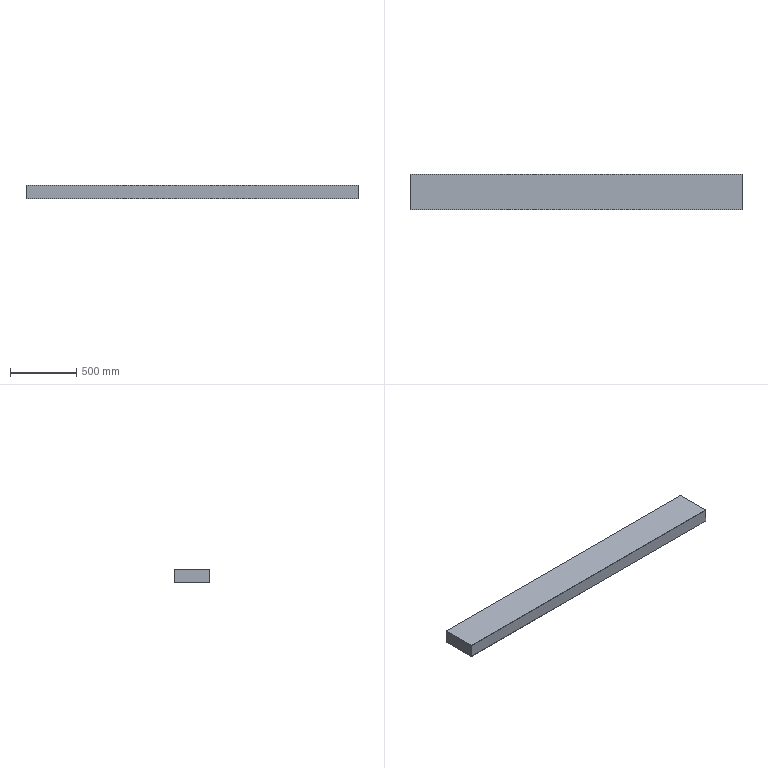Part | STEP file | PN_0037 third-floor site mounting plate 3_Default<As Machined> | 2 solids | 14 faces | box 2515 x 270 x 103 mm | volume 2871750 mm3 | plane 14
STEP:
#1=CARTESIAN_POINT('',(0.,0.,0.));
#2=DIRECTION('',(0.,0.,1.));
#3=DIRECTION('',(1.,0.,0.));
#4=AXIS2_PLACEMENT_3D('',#1,#2,#3);
#5=CARTESIAN_POINT('',(1257.5,-135.,0.));
#6=VERTEX_POINT('',#5);
#7=CARTESIAN_POINT('',(1257.5,135.,0.));
#8=VERTEX_POINT('',#7);
#9=CARTESIAN_POINT('',(1257.5,135.,0.));
#10=DIRECTION('',(0.,1.,0.));
#11=VECTOR('',#10,1.);
#12=LINE('',#9,#11);
#13=CARTESIAN_POINT('',(1257.5,135.,-3.));
#14=DIRECTION('',(1.,0.,0.));
#15=DIRECTION('',(0.,0.,-1.));
#16=AXIS2_PLACEMENT_3D('',#13,#14,#15);
#17=PLANE('',#16);
#18=CARTESIAN_POINT('',(-3.,0.));
#19=DIRECTION('',(0.,1.));
#20=VECTOR('',#19,1.);
#21=LINE('',#18,#20);
#22=(GEOMETRIC_REPRESENTATION_CONTEXT(2)PARAMETRIC_REPRESENTATION_CONTEXT()REPRESENTATION_CONTEXT('',''));
#23=DEFINITIONAL_REPRESENTATION('',(#21),#22);
#24=PCURVE('',#17,#23);
#25=CARTESIAN_POINT('',(0.,0.,0.));
#26=DIRECTION('',(0.,0.,1.));
#27=DIRECTION('',(1.,0.,0.));
#28=AXIS2_PLACEMENT_3D('',#25,#26,#27);
#29=PLANE('',#28);
#30=CARTESIAN_POINT('',(1257.5,135.));
#31=DIRECTION('',(0.,1.));
#32=VECTOR('',#31,1.);
#33=LINE('',#30,#32);
#34=(GEOMETRIC_REPRESENTATION_CONTEXT(2)PARAMETRIC_REPRESENTATION_CONTEXT()REPRESENTATION_CONTEXT('',''));
#35=DEFINITIONAL_REPRESENTATION('',(#33),#34);
#36=PCURVE('',#29,#35);
#37=SURFACE_CURVE('',#12,(#24,#36),.PCURVE_S1.);
#38=EDGE_CURVE('',#6,#8,#37,.T.);
#39=ORIENTED_EDGE('',*,*,#38,.F.);
#40=CARTESIAN_POINT('',(1257.5,-135.,-3.));
#41=VERTEX_POINT('',#40);
#42=CARTESIAN_POINT('',(1257.5,-135.,-3.));
#43=DIRECTION('',(0.,0.,1.));
#44=VECTOR('',#43,1.);
#45=LINE('',#42,#44);
#46=CARTESIAN_POINT('',(0.,-270.));
#47=DIRECTION('',(-1.,0.));
#48=VECTOR('',#47,1.);
#49=LINE('',#46,#48);
#50=(GEOMETRIC_REPRESENTATION_CONTEXT(2)PARAMETRIC_REPRESENTATION_CONTEXT()REPRESENTATION_CONTEXT('',''));
#51=DEFINITIONAL_REPRESENTATION('',(#49),#50);
#52=PCURVE('',#17,#51);
#53=CARTESIAN_POINT('',(-1257.5,-135.,-3.));
#54=DIRECTION('',(0.,-1.,0.));
#55=DIRECTION('',(0.,0.,-1.));
#56=AXIS2_PLACEMENT_3D('',#53,#54,#55);
#57=PLANE('',#56);
#58=CARTESIAN_POINT('',(0.,2515.));
#59=DIRECTION('',(-1.,0.));
#60=VECTOR('',#59,1.);
#61=LINE('',#58,#60);
#62=(GEOMETRIC_REPRESENTATION_CONTEXT(2)PARAMETRIC_REPRESENTATION_CONTEXT()REPRESENTATION_CONTEXT('',''));
#63=DEFINITIONAL_REPRESENTATION('',(#61),#62);
#64=PCURVE('',#57,#63);
#65=SURFACE_CURVE('',#45,(#52,#64),.PCURVE_S1.);
#66=EDGE_CURVE('',#41,#6,#65,.T.);
#67=ORIENTED_EDGE('',*,*,#66,.F.);
#68=CARTESIAN_POINT('',(1257.5,135.,-3.));
#69=VERTEX_POINT('',#68);
#70=CARTESIAN_POINT('',(1257.5,135.,-3.));
#71=DIRECTION('',(0.,1.,0.));
#72=VECTOR('',#71,1.);
#73=LINE('',#70,#72);
#74=CARTESIAN_POINT('',(0.,0.));
#75=DIRECTION('',(0.,1.));
#76=VECTOR('',#75,1.);
#77=LINE('',#74,#76);
#78=(GEOMETRIC_REPRESENTATION_CONTEXT(2)PARAMETRIC_REPRESENTATION_CONTEXT()REPRESENTATION_CONTEXT('',''));
#79=DEFINITIONAL_REPRESENTATION('',(#77),#78);
#80=PCURVE('',#17,#79);
#81=CARTESIAN_POINT('',(0.,0.,-3.));
#82=DIRECTION('',(0.,0.,1.));
#83=DIRECTION('',(1.,0.,0.));
#84=AXIS2_PLACEMENT_3D('',#81,#82,#83);
#85=PLANE('',#84);
#86=CARTESIAN_POINT('',(1257.5,135.));
#87=DIRECTION('',(0.,1.));
#88=VECTOR('',#87,1.);
#89=LINE('',#86,#88);
#90=(GEOMETRIC_REPRESENTATION_CONTEXT(2)PARAMETRIC_REPRESENTATION_CONTEXT()REPRESENTATION_CONTEXT('',''));
#91=DEFINITIONAL_REPRESENTATION('',(#89),#90);
#92=PCURVE('',#85,#91);
#93=SURFACE_CURVE('',#73,(#80,#92),.PCURVE_S1.);
#94=EDGE_CURVE('',#41,#69,#93,.T.);
#95=ORIENTED_EDGE('',*,*,#94,.T.);
#96=CARTESIAN_POINT('',(1257.5,135.,-3.));
#97=DIRECTION('',(0.,0.,1.));
#98=VECTOR('',#97,1.);
#99=LINE('',#96,#98);
#100=CARTESIAN_POINT('',(0.,0.));
#101=DIRECTION('',(-1.,0.));
#102=VECTOR('',#101,1.);
#103=LINE('',#100,#102);
#104=(GEOMETRIC_REPRESENTATION_CONTEXT(2)PARAMETRIC_REPRESENTATION_CONTEXT()REPRESENTATION_CONTEXT('',''));
#105=DEFINITIONAL_REPRESENTATION('',(#103),#104);
#106=PCURVE('',#17,#105);
#107=CARTESIAN_POINT('',(-1257.5,135.,-3.));
#108=DIRECTION('',(0.,1.,0.));
#109=DIRECTION('',(0.,0.,1.));
#110=AXIS2_PLACEMENT_3D('',#107,#108,#109);
#111=PLANE('',#110);
#112=CARTESIAN_POINT('',(0.,2515.));
#113=DIRECTION('',(1.,0.));
#114=VECTOR('',#113,1.);
#115=LINE('',#112,#114);
#116=(GEOMETRIC_REPRESENTATION_CONTEXT(2)PARAMETRIC_REPRESENTATION_CONTEXT()REPRESENTATION_CONTEXT('',''));
#117=DEFINITIONAL_REPRESENTATION('',(#115),#116);
#118=PCURVE('',#111,#117);
#119=SURFACE_CURVE('',#99,(#106,#118),.PCURVE_S1.);
#120=EDGE_CURVE('',#69,#8,#119,.T.);
#121=ORIENTED_EDGE('',*,*,#120,.T.);
#122=EDGE_LOOP('',(#39,#67,#95,#121));
#123=FACE_BOUND('',#122,.T.);
#124=ADVANCED_FACE('',(#123),#17,.T.);
#125=CARTESIAN_POINT('',(-1257.5,-135.,0.));
#126=VERTEX_POINT('',#125);
#127=CARTESIAN_POINT('',(-1257.5,-135.,0.));
#128=DIRECTION('',(1.,0.,0.));
#129=VECTOR('',#128,1.);
#130=LINE('',#127,#129);
#131=CARTESIAN_POINT('',(-3.,0.));
#132=DIRECTION('',(0.,1.));
#133=VECTOR('',#132,1.);
#134=LINE('',#131,#133);
#135=(GEOMETRIC_REPRESENTATION_CONTEXT(2)PARAMETRIC_REPRESENTATION_CONTEXT()REPRESENTATION_CONTEXT('',''));
#136=DEFINITIONAL_REPRESENTATION('',(#134),#135);
#137=PCURVE('',#57,#136);
#138=CARTESIAN_POINT('',(-1257.5,-135.));
#139=DIRECTION('',(1.,0.));
#140=VECTOR('',#139,1.);
#141=LINE('',#138,#140);
#142=(GEOMETRIC_REPRESENTATION_CONTEXT(2)PARAMETRIC_REPRESENTATION_CONTEXT()REPRESENTATION_CONTEXT('',''));
#143=DEFINITIONAL_REPRESENTATION('',(#141),#142);
#144=PCURVE('',#29,#143);
#145=SURFACE_CURVE('',#130,(#137,#144),.PCURVE_S1.);
#146=EDGE_CURVE('',#126,#6,#145,.T.);
#147=ORIENTED_EDGE('',*,*,#146,.F.);
#148=CARTESIAN_POINT('',(-1257.5,-135.,-3.));
#149=VERTEX_POINT('',#148);
#150=CARTESIAN_POINT('',(-1257.5,-135.,-3.));
#151=DIRECTION('',(0.,0.,1.));
#152=VECTOR('',#151,1.);
#153=LINE('',#150,#152);
#154=CARTESIAN_POINT('',(0.,0.));
#155=DIRECTION('',(-1.,0.));
#156=VECTOR('',#155,1.);
#157=LINE('',#154,#156);
#158=(GEOMETRIC_REPRESENTATION_CONTEXT(2)PARAMETRIC_REPRESENTATION_CONTEXT()REPRESENTATION_CONTEXT('',''));
#159=DEFINITIONAL_REPRESENTATION('',(#157),#158);
#160=PCURVE('',#57,#159);
#161=CARTESIAN_POINT('',(-1257.5,135.,-3.));
#162=DIRECTION('',(-1.,0.,0.));
#163=DIRECTION('',(0.,0.,1.));
#164=AXIS2_PLACEMENT_3D('',#161,#162,#163);
#165=PLANE('',#164);
#166=CARTESIAN_POINT('',(0.,-270.));
#167=DIRECTION('',(1.,0.));
#168=VECTOR('',#167,1.);
#169=LINE('',#166,#168);
#170=(GEOMETRIC_REPRESENTATION_CONTEXT(2)PARAMETRIC_REPRESENTATION_CONTEXT()REPRESENTATION_CONTEXT('',''));
#171=DEFINITIONAL_REPRESENTATION('',(#169),#170);
#172=PCURVE('',#165,#171);
#173=SURFACE_CURVE('',#153,(#160,#172),.PCURVE_S1.);
#174=EDGE_CURVE('',#149,#126,#173,.T.);
#175=ORIENTED_EDGE('',*,*,#174,.F.);
#176=CARTESIAN_POINT('',(-1257.5,-135.,-3.));
#177=DIRECTION('',(1.,0.,0.));
#178=VECTOR('',#177,1.);
#179=LINE('',#176,#178);
#180=CARTESIAN_POINT('',(0.,0.));
#181=DIRECTION('',(0.,1.));
#182=VECTOR('',#181,1.);
#183=LINE('',#180,#182);
#184=(GEOMETRIC_REPRESENTATION_CONTEXT(2)PARAMETRIC_REPRESENTATION_CONTEXT()REPRESENTATION_CONTEXT('',''));
#185=DEFINITIONAL_REPRESENTATION('',(#183),#184);
#186=PCURVE('',#57,#185);
#187=CARTESIAN_POINT('',(-1257.5,-135.));
#188=DIRECTION('',(1.,0.));
#189=VECTOR('',#188,1.);
#190=LINE('',#187,#189);
#191=(GEOMETRIC_REPRESENTATION_CONTEXT(2)PARAMETRIC_REPRESENTATION_CONTEXT()REPRESENTATION_CONTEXT('',''));
#192=DEFINITIONAL_REPRESENTATION('',(#190),#191);
#193=PCURVE('',#85,#192);
#194=SURFACE_CURVE('',#179,(#186,#193),.PCURVE_S1.);
#195=EDGE_CURVE('',#149,#41,#194,.T.);
#196=ORIENTED_EDGE('',*,*,#195,.T.);
#197=ORIENTED_EDGE('',*,*,#66,.T.);
#198=EDGE_LOOP('',(#147,#175,#196,#197));
#199=FACE_BOUND('',#198,.T.);
#200=ADVANCED_FACE('',(#199),#57,.T.);
#201=CARTESIAN_POINT('',(-1257.5,135.,0.));
#202=VERTEX_POINT('',#201);
#203=CARTESIAN_POINT('',(-1257.5,135.,0.));
#204=DIRECTION('',(0.,-1.,0.));
#205=VECTOR('',#204,1.);
#206=LINE('',#203,#205);
#207=CARTESIAN_POINT('',(3.,0.));
#208=DIRECTION('',(0.,-1.));
#209=VECTOR('',#208,1.);
#210=LINE('',#207,#209);
#211=(GEOMETRIC_REPRESENTATION_CONTEXT(2)PARAMETRIC_REPRESENTATION_CONTEXT()REPRESENTATION_CONTEXT('',''));
#212=DEFINITIONAL_REPRESENTATION('',(#210),#211);
#213=PCURVE('',#165,#212);
#214=CARTESIAN_POINT('',(-1257.5,135.));
#215=DIRECTION('',(0.,-1.));
#216=VECTOR('',#215,1.);
#217=LINE('',#214,#216);
#218=(GEOMETRIC_REPRESENTATION_CONTEXT(2)PARAMETRIC_REPRESENTATION_CONTEXT()REPRESENTATION_CONTEXT('',''));
#219=DEFINITIONAL_REPRESENTATION('',(#217),#218);
#220=PCURVE('',#29,#219);
#221=SURFACE_CURVE('',#206,(#213,#220),.PCURVE_S1.);
#222=EDGE_CURVE('',#202,#126,#221,.T.);
#223=ORIENTED_EDGE('',*,*,#222,.F.);
#224=CARTESIAN_POINT('',(-1257.5,135.,-3.));
#225=VERTEX_POINT('',#224);
#226=CARTESIAN_POINT('',(-1257.5,135.,-3.));
#227=DIRECTION('',(0.,0.,1.));
#228=VECTOR('',#227,1.);
#229=LINE('',#226,#228);
#230=CARTESIAN_POINT('',(0.,0.));
#231=DIRECTION('',(1.,0.));
#232=VECTOR('',#231,1.);
#233=LINE('',#230,#232);
#234=(GEOMETRIC_REPRESENTATION_CONTEXT(2)PARAMETRIC_REPRESENTATION_CONTEXT()REPRESENTATION_CONTEXT('',''));
#235=DEFINITIONAL_REPRESENTATION('',(#233),#234);
#236=PCURVE('',#165,#235);
#237=CARTESIAN_POINT('',(0.,0.));
#238=DIRECTION('',(1.,0.));
#239=VECTOR('',#238,1.);
#240=LINE('',#237,#239);
#241=(GEOMETRIC_REPRESENTATION_CONTEXT(2)PARAMETRIC_REPRESENTATION_CONTEXT()REPRESENTATION_CONTEXT('',''));
#242=DEFINITIONAL_REPRESENTATION('',(#240),#241);
#243=PCURVE('',#111,#242);
#244=SURFACE_CURVE('',#229,(#236,#243),.PCURVE_S1.);
#245=EDGE_CURVE('',#225,#202,#244,.T.);
#246=ORIENTED_EDGE('',*,*,#245,.F.);
#247=CARTESIAN_POINT('',(-1257.5,135.,-3.));
#248=DIRECTION('',(0.,-1.,0.));
#249=VECTOR('',#248,1.);
#250=LINE('',#247,#249);
#251=CARTESIAN_POINT('',(0.,0.));
#252=DIRECTION('',(0.,-1.));
#253=VECTOR('',#252,1.);
#254=LINE('',#251,#253);
#255=(GEOMETRIC_REPRESENTATION_CONTEXT(2)PARAMETRIC_REPRESENTATION_CONTEXT()REPRESENTATION_CONTEXT('',''));
#256=DEFINITIONAL_REPRESENTATION('',(#254),#255);
#257=PCURVE('',#165,#256);
#258=CARTESIAN_POINT('',(-1257.5,135.));
#259=DIRECTION('',(0.,-1.));
#260=VECTOR('',#259,1.);
#261=LINE('',#258,#260);
#262=(GEOMETRIC_REPRESENTATION_CONTEXT(2)PARAMETRIC_REPRESENTATION_CONTEXT()REPRESENTATION_CONTEXT('',''));
#263=DEFINITIONAL_REPRESENTATION('',(#261),#262);
#264=PCURVE('',#85,#263);
#265=SURFACE_CURVE('',#250,(#257,#264),.PCURVE_S1.);
#266=EDGE_CURVE('',#225,#149,#265,.T.);
#267=ORIENTED_EDGE('',*,*,#266,.T.);
#268=ORIENTED_EDGE('',*,*,#174,.T.);
#269=EDGE_LOOP('',(#223,#246,#267,#268));
#270=FACE_BOUND('',#269,.T.);
#271=ADVANCED_FACE('',(#270),#165,.T.);
#272=CARTESIAN_POINT('',(-1257.5,135.,0.));
#273=DIRECTION('',(-1.,0.,0.));
#274=VECTOR('',#273,1.);
#275=LINE('',#272,#274);
#276=CARTESIAN_POINT('',(3.,0.));
#277=DIRECTION('',(0.,-1.));
#278=VECTOR('',#277,1.);
#279=LINE('',#276,#278);
#280=(GEOMETRIC_REPRESENTATION_CONTEXT(2)PARAMETRIC_REPRESENTATION_CONTEXT()REPRESENTATION_CONTEXT('',''));
#281=DEFINITIONAL_REPRESENTATION('',(#279),#280);
#282=PCURVE('',#111,#281);
#283=CARTESIAN_POINT('',(-1257.5,135.));
#284=DIRECTION('',(-1.,0.));
#285=VECTOR('',#284,1.);
#286=LINE('',#283,#285);
#287=(GEOMETRIC_REPRESENTATION_CONTEXT(2)PARAMETRIC_REPRESENTATION_CONTEXT()REPRESENTATION_CONTEXT('',''));
#288=DEFINITIONAL_REPRESENTATION('',(#286),#287);
#289=PCURVE('',#29,#288);
#290=SURFACE_CURVE('',#275,(#282,#289),.PCURVE_S1.);
#291=EDGE_CURVE('',#8,#202,#290,.T.);
#292=ORIENTED_EDGE('',*,*,#291,.F.);
#293=ORIENTED_EDGE('',*,*,#120,.F.);
#294=CARTESIAN_POINT('',(-1257.5,135.,-3.));
#295=DIRECTION('',(-1.,0.,0.));
#296=VECTOR('',#295,1.);
#297=LINE('',#294,#296);
#298=CARTESIAN_POINT('',(0.,0.));
#299=DIRECTION('',(0.,-1.));
#300=VECTOR('',#299,1.);
#301=LINE('',#298,#300);
#302=(GEOMETRIC_REPRESENTATION_CONTEXT(2)PARAMETRIC_REPRESENTATION_CONTEXT()REPRESENTATION_CONTEXT('',''));
#303=DEFINITIONAL_REPRESENTATION('',(#301),#302);
#304=PCURVE('',#111,#303);
#305=CARTESIAN_POINT('',(-1257.5,135.));
#306=DIRECTION('',(-1.,0.));
#307=VECTOR('',#306,1.);
#308=LINE('',#305,#307);
#309=(GEOMETRIC_REPRESENTATION_CONTEXT(2)PARAMETRIC_REPRESENTATION_CONTEXT()REPRESENTATION_CONTEXT('',''));
#310=DEFINITIONAL_REPRESENTATION('',(#308),#309);
#311=PCURVE('',#85,#310);
#312=SURFACE_CURVE('',#297,(#304,#311),.PCURVE_S1.);
#313=EDGE_CURVE('',#69,#225,#312,.T.);
#314=ORIENTED_EDGE('',*,*,#313,.T.);
#315=ORIENTED_EDGE('',*,*,#245,.T.);
#316=EDGE_LOOP('',(#292,#293,#314,#315));
#317=FACE_BOUND('',#316,.T.);
#318=ADVANCED_FACE('',(#317),#111,.T.);
#319=ORIENTED_EDGE('',*,*,#94,.F.);
#320=ORIENTED_EDGE('',*,*,#195,.F.);
#321=ORIENTED_EDGE('',*,*,#266,.F.);
#322=ORIENTED_EDGE('',*,*,#313,.F.);
#323=EDGE_LOOP('',(#319,#320,#321,#322));
#324=FACE_BOUND('',#323,.T.);
#325=ADVANCED_FACE('',(#324),#85,.F.);
#326=ORIENTED_EDGE('',*,*,#38,.T.);
#327=ORIENTED_EDGE('',*,*,#291,.T.);
#328=ORIENTED_EDGE('',*,*,#222,.T.);
#329=ORIENTED_EDGE('',*,*,#146,.T.);
#330=EDGE_LOOP('',(#326,#327,#328,#329));
#331=FACE_BOUND('',#330,.T.);
#332=ADVANCED_FACE('',(#331),#29,.T.);
#333=CLOSED_SHELL('',(#124,#200,#271,#318,#325,#332));
#334=MANIFOLD_SOLID_BREP('',#333);
#335=CARTESIAN_POINT('',(-1257.5,-135.,-3.));
#336=VERTEX_POINT('',#335);
#337=CARTESIAN_POINT('',(-1257.5,135.,-3.));
#338=VERTEX_POINT('',#337);
#339=CARTESIAN_POINT('',(-1257.5,-135.,-3.));
#340=DIRECTION('',(0.,1.,0.));
#341=VECTOR('',#340,1.);
#342=LINE('',#339,#341);
#343=CARTESIAN_POINT('',(-1257.5,-135.,-103.));
#344=DIRECTION('',(1.,0.,0.));
#345=DIRECTION('',(0.,0.,-1.));
#346=AXIS2_PLACEMENT_3D('',#343,#344,#345);
#347=PLANE('',#346);
#348=CARTESIAN_POINT('',(-100.,0.));
#349=DIRECTION('',(0.,1.));
#350=VECTOR('',#349,1.);
#351=LINE('',#348,#350);
#352=(GEOMETRIC_REPRESENTATION_CONTEXT(2)PARAMETRIC_REPRESENTATION_CONTEXT()REPRESENTATION_CONTEXT('',''));
#353=DEFINITIONAL_REPRESENTATION('',(#351),#352);
#354=PCURVE('',#347,#353);
#355=CARTESIAN_POINT('',(0.,0.,-3.));
#356=DIRECTION('',(0.,0.,1.));
#357=DIRECTION('',(1.,0.,0.));
#358=AXIS2_PLACEMENT_3D('',#355,#356,#357);
#359=PLANE('',#358);
#360=CARTESIAN_POINT('',(-1257.5,-135.));
#361=DIRECTION('',(0.,1.));
#362=VECTOR('',#361,1.);
#363=LINE('',#360,#362);
#364=(GEOMETRIC_REPRESENTATION_CONTEXT(2)PARAMETRIC_REPRESENTATION_CONTEXT()REPRESENTATION_CONTEXT('',''));
#365=DEFINITIONAL_REPRESENTATION('',(#363),#364);
#366=PCURVE('',#359,#365);
#367=SURFACE_CURVE('',#342,(#354,#366),.PCURVE_S1.);
#368=EDGE_CURVE('',#336,#338,#367,.T.);
#369=ORIENTED_EDGE('',*,*,#368,.T.);
#370=CARTESIAN_POINT('',(-1257.5,135.,-103.));
#371=VERTEX_POINT('',#370);
#372=CARTESIAN_POINT('',(-1257.5,135.,-103.));
#373=DIRECTION('',(0.,0.,1.));
#374=VECTOR('',#373,1.);
#375=LINE('',#372,#374);
#376=CARTESIAN_POINT('',(0.,270.));
#377=DIRECTION('',(-1.,0.));
#378=VECTOR('',#377,1.);
#379=LINE('',#376,#378);
#380=(GEOMETRIC_REPRESENTATION_CONTEXT(2)PARAMETRIC_REPRESENTATION_CONTEXT()REPRESENTATION_CONTEXT('',''));
#381=DEFINITIONAL_REPRESENTATION('',(#379),#380);
#382=PCURVE('',#347,#381);
#383=CARTESIAN_POINT('',(-1254.5,135.,-103.));
#384=DIRECTION('',(0.,1.,0.));
#385=DIRECTION('',(0.,0.,1.));
#386=AXIS2_PLACEMENT_3D('',#383,#384,#385);
#387=PLANE('',#386);
#388=CARTESIAN_POINT('',(0.,-3.));
#389=DIRECTION('',(1.,0.));
#390=VECTOR('',#389,1.);
#391=LINE('',#388,#390);
#392=(GEOMETRIC_REPRESENTATION_CONTEXT(2)PARAMETRIC_REPRESENTATION_CONTEXT()REPRESENTATION_CONTEXT('',''));
#393=DEFINITIONAL_REPRESENTATION('',(#391),#392);
#394=PCURVE('',#387,#393);
#395=SURFACE_CURVE('',#375,(#382,#394),.PCURVE_S1.);
#396=EDGE_CURVE('',#371,#338,#395,.T.);
#397=ORIENTED_EDGE('',*,*,#396,.F.);
#398=CARTESIAN_POINT('',(-1257.5,-135.,-103.));
#399=VERTEX_POINT('',#398);
#400=CARTESIAN_POINT('',(-1257.5,-135.,-103.));
#401=DIRECTION('',(0.,1.,0.));
#402=VECTOR('',#401,1.);
#403=LINE('',#400,#402);
#404=CARTESIAN_POINT('',(0.,0.));
#405=DIRECTION('',(0.,1.));
#406=VECTOR('',#405,1.);
#407=LINE('',#404,#406);
#408=(GEOMETRIC_REPRESENTATION_CONTEXT(2)PARAMETRIC_REPRESENTATION_CONTEXT()REPRESENTATION_CONTEXT('',''));
#409=DEFINITIONAL_REPRESENTATION('',(#407),#408);
#410=PCURVE('',#347,#409);
#411=CARTESIAN_POINT('',(0.,0.,-103.));
#412=DIRECTION('',(0.,0.,1.));
#413=DIRECTION('',(1.,0.,0.));
#414=AXIS2_PLACEMENT_3D('',#411,#412,#413);
#415=PLANE('',#414);
#416=CARTESIAN_POINT('',(-1257.5,-135.));
#417=DIRECTION('',(0.,1.));
#418=VECTOR('',#417,1.);
#419=LINE('',#416,#418);
#420=(GEOMETRIC_REPRESENTATION_CONTEXT(2)PARAMETRIC_REPRESENTATION_CONTEXT()REPRESENTATION_CONTEXT('',''));
#421=DEFINITIONAL_REPRESENTATION('',(#419),#420);
#422=PCURVE('',#415,#421);
#423=SURFACE_CURVE('',#403,(#410,#422),.PCURVE_S1.);
#424=EDGE_CURVE('',#399,#371,#423,.T.);
#425=ORIENTED_EDGE('',*,*,#424,.F.);
#426=CARTESIAN_POINT('',(-1257.5,-135.,-103.));
#427=DIRECTION('',(0.,0.,1.));
#428=VECTOR('',#427,1.);
#429=LINE('',#426,#428);
#430=CARTESIAN_POINT('',(0.,0.));
#431=DIRECTION('',(-1.,0.));
#432=VECTOR('',#431,1.);
#433=LINE('',#430,#432);
#434=(GEOMETRIC_REPRESENTATION_CONTEXT(2)PARAMETRIC_REPRESENTATION_CONTEXT()REPRESENTATION_CONTEXT('',''));
#435=DEFINITIONAL_REPRESENTATION('',(#433),#434);
#436=PCURVE('',#347,#435);
#437=CARTESIAN_POINT('',(1257.5,-135.,-103.));
#438=DIRECTION('',(0.,1.,0.));
#439=DIRECTION('',(0.,0.,1.));
#440=AXIS2_PLACEMENT_3D('',#437,#438,#439);
#441=PLANE('',#440);
#442=CARTESIAN_POINT('',(0.,-2515.));
#443=DIRECTION('',(1.,0.));
#444=VECTOR('',#443,1.);
#445=LINE('',#442,#444);
#446=(GEOMETRIC_REPRESENTATION_CONTEXT(2)PARAMETRIC_REPRESENTATION_CONTEXT()REPRESENTATION_CONTEXT('',''));
#447=DEFINITIONAL_REPRESENTATION('',(#445),#446);
#448=PCURVE('',#441,#447);
#449=SURFACE_CURVE('',#429,(#436,#448),.PCURVE_S1.);
#450=EDGE_CURVE('',#399,#336,#449,.T.);
#451=ORIENTED_EDGE('',*,*,#450,.T.);
#452=EDGE_LOOP('',(#369,#397,#425,#451));
#453=FACE_BOUND('',#452,.T.);
#454=ADVANCED_FACE('',(#453),#347,.F.);
#455=CARTESIAN_POINT('',(-1254.5,135.,-3.));
#456=VERTEX_POINT('',#455);
#457=CARTESIAN_POINT('',(-1254.5,135.,-3.));
#458=DIRECTION('',(-1.,0.,0.));
#459=VECTOR('',#458,1.);
#460=LINE('',#457,#459);
#461=CARTESIAN_POINT('',(100.,0.));
#462=DIRECTION('',(0.,-1.));
#463=VECTOR('',#462,1.);
#464=LINE('',#461,#463);
#465=(GEOMETRIC_REPRESENTATION_CONTEXT(2)PARAMETRIC_REPRESENTATION_CONTEXT()REPRESENTATION_CONTEXT('',''));
#466=DEFINITIONAL_REPRESENTATION('',(#464),#465);
#467=PCURVE('',#387,#466);
#468=CARTESIAN_POINT('',(-1254.5,135.));
#469=DIRECTION('',(-1.,0.));
#470=VECTOR('',#469,1.);
#471=LINE('',#468,#470);
#472=(GEOMETRIC_REPRESENTATION_CONTEXT(2)PARAMETRIC_REPRESENTATION_CONTEXT()REPRESENTATION_CONTEXT('',''));
#473=DEFINITIONAL_REPRESENTATION('',(#471),#472);
#474=PCURVE('',#359,#473);
#475=SURFACE_CURVE('',#460,(#467,#474),.PCURVE_S1.);
#476=EDGE_CURVE('',#456,#338,#475,.T.);
#477=ORIENTED_EDGE('',*,*,#476,.F.);
#478=CARTESIAN_POINT('',(-1254.5,135.,-103.));
#479=VERTEX_POINT('',#478);
#480=CARTESIAN_POINT('',(-1254.5,135.,-103.));
#481=DIRECTION('',(0.,0.,1.));
#482=VECTOR('',#481,1.);
#483=LINE('',#480,#482);
#484=CARTESIAN_POINT('',(0.,0.));
#485=DIRECTION('',(1.,0.));
#486=VECTOR('',#485,1.);
#487=LINE('',#484,#486);
#488=(GEOMETRIC_REPRESENTATION_CONTEXT(2)PARAMETRIC_REPRESENTATION_CONTEXT()REPRESENTATION_CONTEXT('',''));
#489=DEFINITIONAL_REPRESENTATION('',(#487),#488);
#490=PCURVE('',#387,#489);
#491=CARTESIAN_POINT('',(-1254.5,-135.,-103.));
#492=DIRECTION('',(1.,0.,0.));
#493=DIRECTION('',(0.,0.,-1.));
#494=AXIS2_PLACEMENT_3D('',#491,#492,#493);
#495=PLANE('',#494);
#496=CARTESIAN_POINT('',(0.,270.));
#497=DIRECTION('',(-1.,0.));
#498=VECTOR('',#497,1.);
#499=LINE('',#496,#498);
#500=(GEOMETRIC_REPRESENTATION_CONTEXT(2)PARAMETRIC_REPRESENTATION_CONTEXT()REPRESENTATION_CONTEXT('',''));
#501=DEFINITIONAL_REPRESENTATION('',(#499),#500);
#502=PCURVE('',#495,#501);
#503=SURFACE_CURVE('',#483,(#490,#502),.PCURVE_S1.);
#504=EDGE_CURVE('',#479,#456,#503,.T.);
#505=ORIENTED_EDGE('',*,*,#504,.F.);
#506=CARTESIAN_POINT('',(-1254.5,135.,-103.));
#507=DIRECTION('',(-1.,0.,0.));
#508=VECTOR('',#507,1.);
#509=LINE('',#506,#508);
#510=CARTESIAN_POINT('',(0.,0.));
#511=DIRECTION('',(0.,-1.));
#512=VECTOR('',#511,1.);
#513=LINE('',#510,#512);
#514=(GEOMETRIC_REPRESENTATION_CONTEXT(2)PARAMETRIC_REPRESENTATION_CONTEXT()REPRESENTATION_CONTEXT('',''));
#515=DEFINITIONAL_REPRESENTATION('',(#513),#514);
#516=PCURVE('',#387,#515);
#517=CARTESIAN_POINT('',(-1254.5,135.));
#518=DIRECTION('',(-1.,0.));
#519=VECTOR('',#518,1.);
#520=LINE('',#517,#519);
#521=(GEOMETRIC_REPRESENTATION_CONTEXT(2)PARAMETRIC_REPRESENTATION_CONTEXT()REPRESENTATION_CONTEXT('',''));
#522=DEFINITIONAL_REPRESENTATION('',(#520),#521);
#523=PCURVE('',#415,#522);
#524=SURFACE_CURVE('',#509,(#516,#523),.PCURVE_S1.);
#525=EDGE_CURVE('',#479,#371,#524,.T.);
#526=ORIENTED_EDGE('',*,*,#525,.T.);
#527=ORIENTED_EDGE('',*,*,#396,.T.);
#528=EDGE_LOOP('',(#477,#505,#526,#527));
#529=FACE_BOUND('',#528,.T.);
#530=ADVANCED_FACE('',(#529),#387,.T.);
#531=CARTESIAN_POINT('',(-1254.5,-132.,-3.));
#532=VERTEX_POINT('',#531);
#533=CARTESIAN_POINT('',(-1254.5,-135.,-3.));
#534=DIRECTION('',(0.,1.,0.));
#535=VECTOR('',#534,1.);
#536=LINE('',#533,#535);
#537=CARTESIAN_POINT('',(-100.,0.));
#538=DIRECTION('',(0.,1.));
#539=VECTOR('',#538,1.);
#540=LINE('',#537,#539);
#541=(GEOMETRIC_REPRESENTATION_CONTEXT(2)PARAMETRIC_REPRESENTATION_CONTEXT()REPRESENTATION_CONTEXT('',''));
#542=DEFINITIONAL_REPRESENTATION('',(#540),#541);
#543=PCURVE('',#495,#542);
#544=CARTESIAN_POINT('',(-1254.5,-135.));
#545=DIRECTION('',(0.,1.));
#546=VECTOR('',#545,1.);
#547=LINE('',#544,#546);
#548=(GEOMETRIC_REPRESENTATION_CONTEXT(2)PARAMETRIC_REPRESENTATION_CONTEXT()REPRESENTATION_CONTEXT('',''));
#549=DEFINITIONAL_REPRESENTATION('',(#547),#548);
#550=PCURVE('',#359,#549);
#551=SURFACE_CURVE('',#536,(#543,#550),.PCURVE_S1.);
#552=EDGE_CURVE('',#532,#456,#551,.T.);
#553=ORIENTED_EDGE('',*,*,#552,.F.);
#554=CARTESIAN_POINT('',(-1254.5,-132.,-103.));
#555=VERTEX_POINT('',#554);
#556=CARTESIAN_POINT('',(-1254.5,-132.,-103.));
#557=DIRECTION('',(0.,0.,1.));
#558=VECTOR('',#557,1.);
#559=LINE('',#556,#558);
#560=CARTESIAN_POINT('',(0.,3.));
#561=DIRECTION('',(-1.,0.));
#562=VECTOR('',#561,1.);
#563=LINE('',#560,#562);
#564=(GEOMETRIC_REPRESENTATION_CONTEXT(2)PARAMETRIC_REPRESENTATION_CONTEXT()REPRESENTATION_CONTEXT('',''));
#565=DEFINITIONAL_REPRESENTATION('',(#563),#564);
#566=PCURVE('',#495,#565);
#567=CARTESIAN_POINT('',(1257.5,-132.,-103.));
#568=DIRECTION('',(0.,1.,0.));
#569=DIRECTION('',(0.,0.,1.));
#570=AXIS2_PLACEMENT_3D('',#567,#568,#569);
#571=PLANE('',#570);
#572=CARTESIAN_POINT('',(0.,-2512.));
#573=DIRECTION('',(1.,0.));
#574=VECTOR('',#573,1.);
#575=LINE('',#572,#574);
#576=(GEOMETRIC_REPRESENTATION_CONTEXT(2)PARAMETRIC_REPRESENTATION_CONTEXT()REPRESENTATION_CONTEXT('',''));
#577=DEFINITIONAL_REPRESENTATION('',(#575),#576);
#578=PCURVE('',#571,#577);
#579=SURFACE_CURVE('',#559,(#566,#578),.PCURVE_S1.);
#580=EDGE_CURVE('',#555,#532,#579,.T.);
#581=ORIENTED_EDGE('',*,*,#580,.F.);
#582=CARTESIAN_POINT('',(-1254.5,-135.,-103.));
#583=DIRECTION('',(0.,1.,0.));
#584=VECTOR('',#583,1.);
#585=LINE('',#582,#584);
#586=CARTESIAN_POINT('',(0.,0.));
#587=DIRECTION('',(0.,1.));
#588=VECTOR('',#587,1.);
#589=LINE('',#586,#588);
#590=(GEOMETRIC_REPRESENTATION_CONTEXT(2)PARAMETRIC_REPRESENTATION_CONTEXT()REPRESENTATION_CONTEXT('',''));
#591=DEFINITIONAL_REPRESENTATION('',(#589),#590);
#592=PCURVE('',#495,#591);
#593=CARTESIAN_POINT('',(-1254.5,-135.));
#594=DIRECTION('',(0.,1.));
#595=VECTOR('',#594,1.);
#596=LINE('',#593,#595);
#597=(GEOMETRIC_REPRESENTATION_CONTEXT(2)PARAMETRIC_REPRESENTATION_CONTEXT()REPRESENTATION_CONTEXT('',''));
#598=DEFINITIONAL_REPRESENTATION('',(#596),#597);
#599=PCURVE('',#415,#598);
#600=SURFACE_CURVE('',#585,(#592,#599),.PCURVE_S1.);
#601=EDGE_CURVE('',#555,#479,#600,.T.);
#602=ORIENTED_EDGE('',*,*,#601,.T.);
#603=ORIENTED_EDGE('',*,*,#504,.T.);
#604=EDGE_LOOP('',(#553,#581,#602,#603));
#605=FACE_BOUND('',#604,.T.);
#606=ADVANCED_FACE('',(#605),#495,.T.);
#607=CARTESIAN_POINT('',(1257.5,-132.,-3.));
#608=VERTEX_POINT('',#607);
#609=CARTESIAN_POINT('',(1257.5,-132.,-3.));
#610=DIRECTION('',(-1.,0.,0.));
#611=VECTOR('',#610,1.);
#612=LINE('',#609,#611);
#613=CARTESIAN_POINT('',(100.,0.));
#614=DIRECTION('',(0.,-1.));
#615=VECTOR('',#614,1.);
#616=LINE('',#613,#615);
#617=(GEOMETRIC_REPRESENTATION_CONTEXT(2)PARAMETRIC_REPRESENTATION_CONTEXT()REPRESENTATION_CONTEXT('',''));
#618=DEFINITIONAL_REPRESENTATION('',(#616),#617);
#619=PCURVE('',#571,#618);
#620=CARTESIAN_POINT('',(1257.5,-132.));
#621=DIRECTION('',(-1.,0.));
#622=VECTOR('',#621,1.);
#623=LINE('',#620,#622);
#624=(GEOMETRIC_REPRESENTATION_CONTEXT(2)PARAMETRIC_REPRESENTATION_CONTEXT()REPRESENTATION_CONTEXT('',''));
#625=DEFINITIONAL_REPRESENTATION('',(#623),#624);
#626=PCURVE('',#359,#625);
#627=SURFACE_CURVE('',#612,(#619,#626),.PCURVE_S1.);
#628=EDGE_CURVE('',#608,#532,#627,.T.);
#629=ORIENTED_EDGE('',*,*,#628,.F.);
#630=CARTESIAN_POINT('',(1257.5,-132.,-103.));
#631=VERTEX_POINT('',#630);
#632=CARTESIAN_POINT('',(1257.5,-132.,-103.));
#633=DIRECTION('',(0.,0.,1.));
#634=VECTOR('',#633,1.);
#635=LINE('',#632,#634);
#636=CARTESIAN_POINT('',(0.,0.));
#637=DIRECTION('',(1.,0.));
#638=VECTOR('',#637,1.);
#639=LINE('',#636,#638);
#640=(GEOMETRIC_REPRESENTATION_CONTEXT(2)PARAMETRIC_REPRESENTATION_CONTEXT()REPRESENTATION_CONTEXT('',''));
#641=DEFINITIONAL_REPRESENTATION('',(#639),#640);
#642=PCURVE('',#571,#641);
#643=CARTESIAN_POINT('',(1257.5,-135.,-103.));
#644=DIRECTION('',(1.,0.,0.));
#645=DIRECTION('',(0.,0.,-1.));
#646=AXIS2_PLACEMENT_3D('',#643,#644,#645);
#647=PLANE('',#646);
#648=CARTESIAN_POINT('',(0.,3.));
#649=DIRECTION('',(-1.,0.));
#650=VECTOR('',#649,1.);
#651=LINE('',#648,#650);
#652=(GEOMETRIC_REPRESENTATION_CONTEXT(2)PARAMETRIC_REPRESENTATION_CONTEXT()REPRESENTATION_CONTEXT('',''));
#653=DEFINITIONAL_REPRESENTATION('',(#651),#652);
#654=PCURVE('',#647,#653);
#655=SURFACE_CURVE('',#635,(#642,#654),.PCURVE_S1.);
#656=EDGE_CURVE('',#631,#608,#655,.T.);
#657=ORIENTED_EDGE('',*,*,#656,.F.);
#658=CARTESIAN_POINT('',(1257.5,-132.,-103.));
#659=DIRECTION('',(-1.,0.,0.));
#660=VECTOR('',#659,1.);
#661=LINE('',#658,#660);
#662=CARTESIAN_POINT('',(0.,0.));
#663=DIRECTION('',(0.,-1.));
#664=VECTOR('',#663,1.);
#665=LINE('',#662,#664);
#666=(GEOMETRIC_REPRESENTATION_CONTEXT(2)PARAMETRIC_REPRESENTATION_CONTEXT()REPRESENTATION_CONTEXT('',''));
#667=DEFINITIONAL_REPRESENTATION('',(#665),#666);
#668=PCURVE('',#571,#667);
#669=CARTESIAN_POINT('',(1257.5,-132.));
#670=DIRECTION('',(-1.,0.));
#671=VECTOR('',#670,1.);
#672=LINE('',#669,#671);
#673=(GEOMETRIC_REPRESENTATION_CONTEXT(2)PARAMETRIC_REPRESENTATION_CONTEXT()REPRESENTATION_CONTEXT('',''));
#674=DEFINITIONAL_REPRESENTATION('',(#672),#673);
#675=PCURVE('',#415,#674);
#676=SURFACE_CURVE('',#661,(#668,#675),.PCURVE_S1.);
#677=EDGE_CURVE('',#631,#555,#676,.T.);
#678=ORIENTED_EDGE('',*,*,#677,.T.);
#679=ORIENTED_EDGE('',*,*,#580,.T.);
#680=EDGE_LOOP('',(#629,#657,#678,#679));
#681=FACE_BOUND('',#680,.T.);
#682=ADVANCED_FACE('',(#681),#571,.T.);
#683=CARTESIAN_POINT('',(1257.5,-135.,-3.));
#684=VERTEX_POINT('',#683);
#685=CARTESIAN_POINT('',(1257.5,-135.,-3.));
#686=DIRECTION('',(0.,1.,0.));
#687=VECTOR('',#686,1.);
#688=LINE('',#685,#687);
#689=CARTESIAN_POINT('',(-100.,0.));
#690=DIRECTION('',(0.,1.));
#691=VECTOR('',#690,1.);
#692=LINE('',#689,#691);
#693=(GEOMETRIC_REPRESENTATION_CONTEXT(2)PARAMETRIC_REPRESENTATION_CONTEXT()REPRESENTATION_CONTEXT('',''));
#694=DEFINITIONAL_REPRESENTATION('',(#692),#693);
#695=PCURVE('',#647,#694);
#696=CARTESIAN_POINT('',(1257.5,-135.));
#697=DIRECTION('',(0.,1.));
#698=VECTOR('',#697,1.);
#699=LINE('',#696,#698);
#700=(GEOMETRIC_REPRESENTATION_CONTEXT(2)PARAMETRIC_REPRESENTATION_CONTEXT()REPRESENTATION_CONTEXT('',''));
#701=DEFINITIONAL_REPRESENTATION('',(#699),#700);
#702=PCURVE('',#359,#701);
#703=SURFACE_CURVE('',#688,(#695,#702),.PCURVE_S1.);
#704=EDGE_CURVE('',#684,#608,#703,.T.);
#705=ORIENTED_EDGE('',*,*,#704,.F.);
#706=CARTESIAN_POINT('',(1257.5,-135.,-103.));
#707=VERTEX_POINT('',#706);
#708=CARTESIAN_POINT('',(1257.5,-135.,-103.));
#709=DIRECTION('',(0.,0.,1.));
#710=VECTOR('',#709,1.);
#711=LINE('',#708,#710);
#712=CARTESIAN_POINT('',(0.,0.));
#713=DIRECTION('',(-1.,0.));
#714=VECTOR('',#713,1.);
#715=LINE('',#712,#714);
#716=(GEOMETRIC_REPRESENTATION_CONTEXT(2)PARAMETRIC_REPRESENTATION_CONTEXT()REPRESENTATION_CONTEXT('',''));
#717=DEFINITIONAL_REPRESENTATION('',(#715),#716);
#718=PCURVE('',#647,#717);
#719=CARTESIAN_POINT('',(0.,0.));
#720=DIRECTION('',(1.,0.));
#721=VECTOR('',#720,1.);
#722=LINE('',#719,#721);
#723=(GEOMETRIC_REPRESENTATION_CONTEXT(2)PARAMETRIC_REPRESENTATION_CONTEXT()REPRESENTATION_CONTEXT('',''));
#724=DEFINITIONAL_REPRESENTATION('',(#722),#723);
#725=PCURVE('',#441,#724);
#726=SURFACE_CURVE('',#711,(#718,#725),.PCURVE_S1.);
#727=EDGE_CURVE('',#707,#684,#726,.T.);
#728=ORIENTED_EDGE('',*,*,#727,.F.);
#729=CARTESIAN_POINT('',(1257.5,-135.,-103.));
#730=DIRECTION('',(0.,1.,0.));
#731=VECTOR('',#730,1.);
#732=LINE('',#729,#731);
#733=CARTESIAN_POINT('',(0.,0.));
#734=DIRECTION('',(0.,1.));
#735=VECTOR('',#734,1.);
#736=LINE('',#733,#735);
#737=(GEOMETRIC_REPRESENTATION_CONTEXT(2)PARAMETRIC_REPRESENTATION_CONTEXT()REPRESENTATION_CONTEXT('',''));
#738=DEFINITIONAL_REPRESENTATION('',(#736),#737);
#739=PCURVE('',#647,#738);
#740=CARTESIAN_POINT('',(1257.5,-135.));
#741=DIRECTION('',(0.,1.));
#742=VECTOR('',#741,1.);
#743=LINE('',#740,#742);
#744=(GEOMETRIC_REPRESENTATION_CONTEXT(2)PARAMETRIC_REPRESENTATION_CONTEXT()REPRESENTATION_CONTEXT('',''));
#745=DEFINITIONAL_REPRESENTATION('',(#743),#744);
#746=PCURVE('',#415,#745);
#747=SURFACE_CURVE('',#732,(#739,#746),.PCURVE_S1.);
#748=EDGE_CURVE('',#707,#631,#747,.T.);
#749=ORIENTED_EDGE('',*,*,#748,.T.);
#750=ORIENTED_EDGE('',*,*,#656,.T.);
#751=EDGE_LOOP('',(#705,#728,#749,#750));
#752=FACE_BOUND('',#751,.T.);
#753=ADVANCED_FACE('',(#752),#647,.T.);
#754=CARTESIAN_POINT('',(1257.5,-135.,-3.));
#755=DIRECTION('',(-1.,0.,0.));
#756=VECTOR('',#755,1.);
#757=LINE('',#754,#756);
#758=CARTESIAN_POINT('',(100.,0.));
#759=DIRECTION('',(0.,-1.));
#760=VECTOR('',#759,1.);
#761=LINE('',#758,#760);
#762=(GEOMETRIC_REPRESENTATION_CONTEXT(2)PARAMETRIC_REPRESENTATION_CONTEXT()REPRESENTATION_CONTEXT('',''));
#763=DEFINITIONAL_REPRESENTATION('',(#761),#762);
#764=PCURVE('',#441,#763);
#765=CARTESIAN_POINT('',(1257.5,-135.));
#766=DIRECTION('',(-1.,0.));
#767=VECTOR('',#766,1.);
#768=LINE('',#765,#767);
#769=(GEOMETRIC_REPRESENTATION_CONTEXT(2)PARAMETRIC_REPRESENTATION_CONTEXT()REPRESENTATION_CONTEXT('',''));
#770=DEFINITIONAL_REPRESENTATION('',(#768),#769);
#771=PCURVE('',#359,#770);
#772=SURFACE_CURVE('',#757,(#764,#771),.PCURVE_S1.);
#773=EDGE_CURVE('',#684,#336,#772,.T.);
#774=ORIENTED_EDGE('',*,*,#773,.T.);
#775=ORIENTED_EDGE('',*,*,#450,.F.);
#776=CARTESIAN_POINT('',(1257.5,-135.,-103.));
#777=DIRECTION('',(-1.,0.,0.));
#778=VECTOR('',#777,1.);
#779=LINE('',#776,#778);
#780=CARTESIAN_POINT('',(0.,0.));
#781=DIRECTION('',(0.,-1.));
#782=VECTOR('',#781,1.);
#783=LINE('',#780,#782);
#784=(GEOMETRIC_REPRESENTATION_CONTEXT(2)PARAMETRIC_REPRESENTATION_CONTEXT()REPRESENTATION_CONTEXT('',''));
#785=DEFINITIONAL_REPRESENTATION('',(#783),#784);
#786=PCURVE('',#441,#785);
#787=CARTESIAN_POINT('',(1257.5,-135.));
#788=DIRECTION('',(-1.,0.));
#789=VECTOR('',#788,1.);
#790=LINE('',#787,#789);
#791=(GEOMETRIC_REPRESENTATION_CONTEXT(2)PARAMETRIC_REPRESENTATION_CONTEXT()REPRESENTATION_CONTEXT('',''));
#792=DEFINITIONAL_REPRESENTATION('',(#790),#791);
#793=PCURVE('',#415,#792);
#794=SURFACE_CURVE('',#779,(#786,#793),.PCURVE_S1.);
#795=EDGE_CURVE('',#707,#399,#794,.T.);
#796=ORIENTED_EDGE('',*,*,#795,.F.);
#797=ORIENTED_EDGE('',*,*,#727,.T.);
#798=EDGE_LOOP('',(#774,#775,#796,#797));
#799=FACE_BOUND('',#798,.T.);
#800=ADVANCED_FACE('',(#799),#441,.F.);
#801=ORIENTED_EDGE('',*,*,#424,.T.);
#802=ORIENTED_EDGE('',*,*,#525,.F.);
#803=ORIENTED_EDGE('',*,*,#601,.F.);
#804=ORIENTED_EDGE('',*,*,#677,.F.);
#805=ORIENTED_EDGE('',*,*,#748,.F.);
#806=ORIENTED_EDGE('',*,*,#795,.T.);
#807=EDGE_LOOP('',(#801,#802,#803,#804,#805,#806));
#808=FACE_BOUND('',#807,.T.);
#809=ADVANCED_FACE('',(#808),#415,.F.);
#810=ORIENTED_EDGE('',*,*,#368,.F.);
#811=ORIENTED_EDGE('',*,*,#773,.F.);
#812=ORIENTED_EDGE('',*,*,#704,.T.);
#813=ORIENTED_EDGE('',*,*,#628,.T.);
#814=ORIENTED_EDGE('',*,*,#552,.T.);
#815=ORIENTED_EDGE('',*,*,#476,.T.);
#816=EDGE_LOOP('',(#810,#811,#812,#813,#814,#815));
#817=FACE_BOUND('',#816,.T.);
#818=ADVANCED_FACE('',(#817),#359,.T.);
#819=CLOSED_SHELL('',(#454,#530,#606,#682,#753,#800,#809,#818));
#820=MANIFOLD_SOLID_BREP('',#819);
#821=(LENGTH_UNIT()NAMED_UNIT(*)SI_UNIT(.MILLI.,.METRE.));
#822=UNCERTAINTY_MEASURE_WITH_UNIT(LENGTH_MEASURE(0.0000001),#821,'','');
#823=(NAMED_UNIT(*)PLANE_ANGLE_UNIT()SI_UNIT($,.RADIAN.));
#824=(NAMED_UNIT(*)SI_UNIT($,.STERADIAN.)SOLID_ANGLE_UNIT());
#825=(GEOMETRIC_REPRESENTATION_CONTEXT(3)GLOBAL_UNCERTAINTY_ASSIGNED_CONTEXT((#822))GLOBAL_UNIT_ASSIGNED_CONTEXT((#821,#823,#824))REPRESENTATION_CONTEXT('',''));
#826=SHAPE_REPRESENTATION('',(#4,#334,#820),#825);